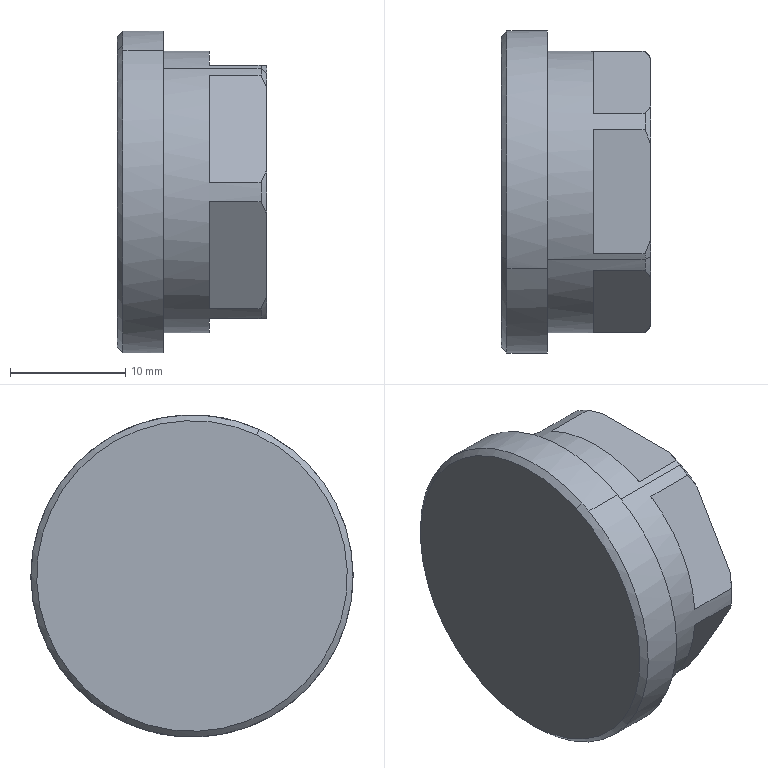Part | STEP file | Joint.1.stp | 1 solid | 34 faces | box 13 x 28 x 28 mm | volume 4907 mm3 | plane 17 | cone 9 | cylinder 8 | commonest cylinder face diameters 15 x2 17 x2 24.5 x2 28 x2